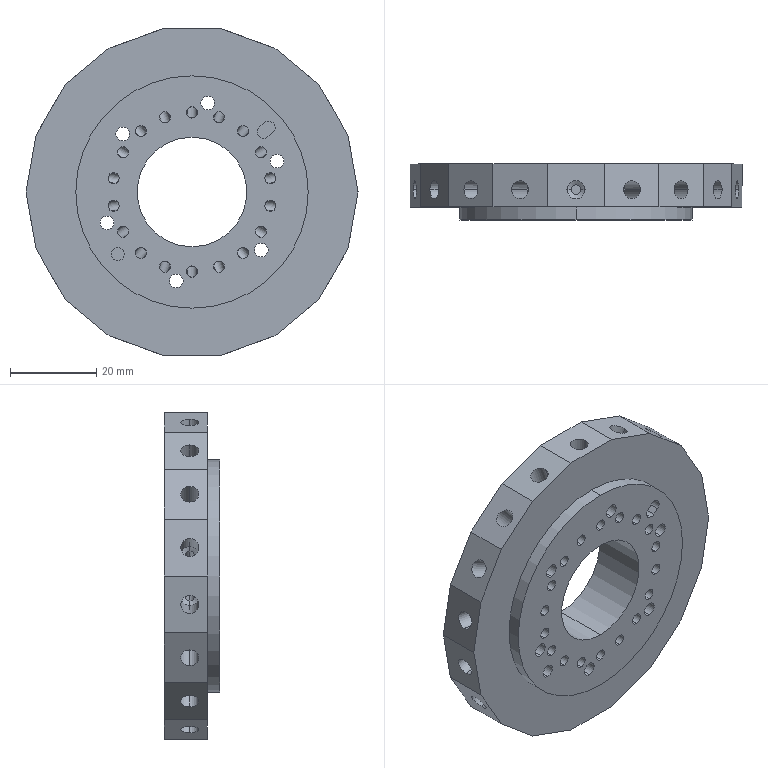Part | SolidWorks | features ICE 12, CirPattern 5, HoleWzd 2, 3DProfileFeature 1, Chamfer 1, Cut 1, Extrusion 1 | 1 solid | 308 faces | box 77.172 x 13 x 76 mm | volume 40512 mm3 | cylinder 175 | plane 89 | cone 44 | commonest cylinder face diameters 2.3 x54 2.6 x36 4.2 x36 3.2 x12 7 x12 2.5 x8